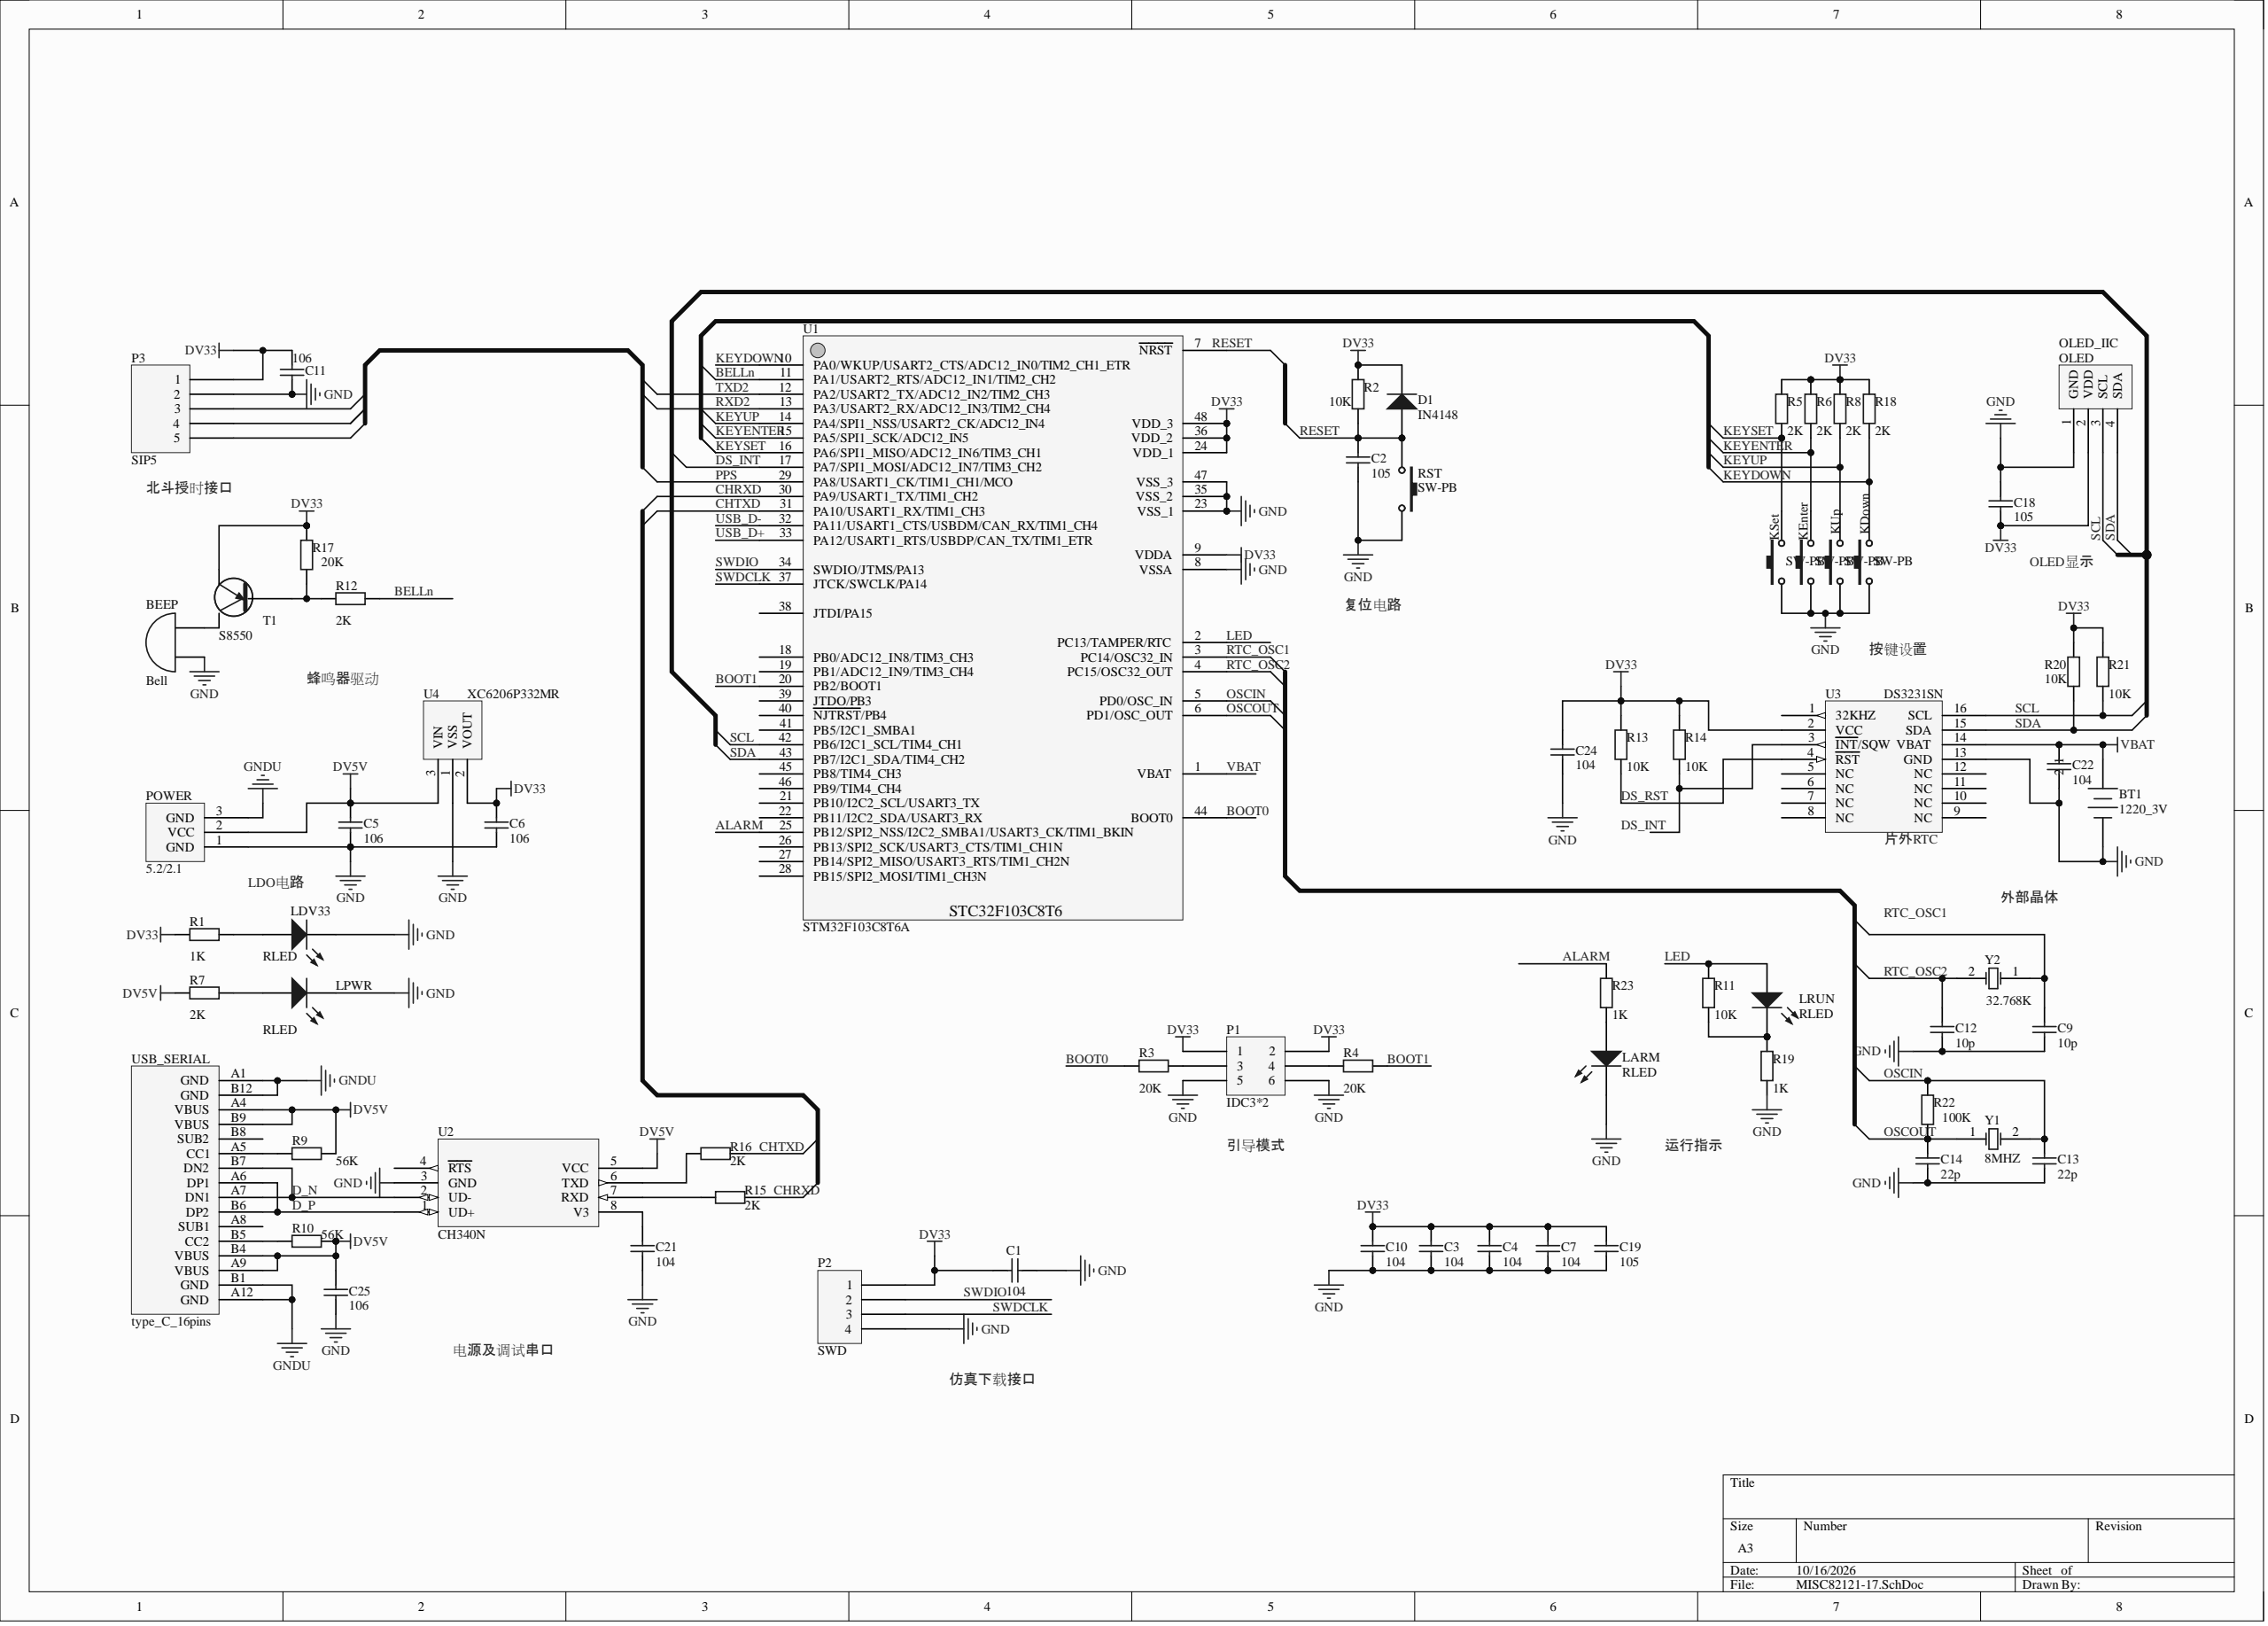Circuit board | Altium Designer | 67 parts | 42 nets
Bill of materials:
Comment,Description,Designator,Footprint,LibRef,Quantity
"Bell","Electrical Bell","BEEP","HN9650B","Bell","1"
"1220_3V","Multicell Battery","BT1","CR1220","Battery","1"
"104","Capacitor","C1, C3, C4, C7, C10, C21, C22, C24","C0805","Cap","8"
"105","Capacitor","C2, C19","C0805","Cap","2"
"106","Capacitor","C5, C6, C11","C0805","Cap","3"
"10p","Capacitor","C9, C12","C0603","Cap","2"
"22p","Capacitor","C13, C14","C0603","Cap","2"
"IN4148","Default Diode","D1","D0805","Diode","1"
"SW-PB","Switch","KDown, KEnter, KSet, KUp, RST","KEY_8mm","SW-PB","5"
"RLED","Typical INFRARED GaAs LED","LARM, LDV33, LPWR, LRUN","LED0805","LED0","4"
"OLED_IIC","","OLED","OLED","OLED_I2C_I2164","1"
"IDC3*2","","P1","HDR2X3","IDC3*2","1"
"SWD","","P2","HDR1X4","SWD","1"
"SIP5","","P3","HDR1X5","SIP5","1"
"5.2/2.1","","POWER","SWC_SET","5.2/2.1","1"
"Res2","Resistor","R1, R2, R3, R4, R5, R6, R7, R8, R9, R10, R11, R12, R13, R14, R15, R16, R17, R18, R19, R20, R21, R22, R23","R0805","Res2","23"
"S8550","","T1","SOT-23","S8550","1"
"STM32F103C8T6A","","U1","LQFP48","STM32F103C8T6","1"
"CH340N","","U2","SO-8","CH340N","1"
"DS3231SN","","U3","SOP-16","DS3231SN","1"
"XC6206P332MR","","U4","SOT-23S","XC6206P332MR","1"
"type_C_16pins","","USB_SERIAL","TYPE_C_16PIN","type_C_16pins","1"
"8MHZ","Crystal Oscillator","Y1","OSC 5032-2P","XTAL","1"
"32.768K","Crystal Oscillator","Y2","OSC_2*6","XTAL","1"
Netlist (Protel format):
[
BEEP
HN9650B
Bell



]
[
BT1
CR1220
1220_3V



]
[
C1
C0805
104



]
[
C2
C0805
105



]
[
C3
C0805
104



]
[
C4
C0805
104



]
[
C5
C0805
106



]
[
C6
C0805
106



]
[
C7
C0805
104



]
[
C9
C0603
10p



]
[
C10
C0805
104



]
[
C11
C0805
106



]
[
C12
C0603
10p



]
[
C13
C0603
22p



]
[
C14
C0603
22p



]
[
C18
C0805
105



]
[
C19
C0805
105



]
[
C21
C0805
104



]
[
C22
C0805
104



]
[
C24
C0805
104



]
[
C25
C0805
106



]
[
D1
D0805
IN4148



]
[
KDown
KEY_8mm
SW-PB



]
[
KEnter
KEY_8mm
SW-PB



]
[
KSet
KEY_8mm
SW-PB



]
[
KUp
KEY_8mm
SW-PB



]
[
LARM
LED0805
RLED



]
[
LDV33
LED0805
RLED



]
[
LPWR
LED0805
RLED



]
[
LRUN
LED0805
RLED



]
[
OLED
OLED
OLED_IIC



]
[
P1
HDR2X3
IDC3*2



]
[
P2
HDR1X4
SWD



]
[
P3
HDR1X5
SIP5



]
[
POWER
SWC_SET
5.2/2.1



]
[
R1
R0805
Res2



]
[
R2
R0805
Res2



]
[
R3
R0805
Res2



]
[
R4
R0805
Res2



]
[
R5
R0805
Res2



]
[
R6
R0805
Res2



]
[
R7
R0805
Res2



]
[
R8
R0805
Res2



]
[
R9
R0805
Res2



]
[
R10
R0805
Res2



]
[
R11
R0805
Res2



]
[
R12
R0805
Res2



]
[
R13
R0805
Res2



]
[
R14
R0805
Res2



]
[
R15
R0805
Res2



]
[
R16
R0805
Res2



]
[
R17
R0805
Res2



]
[
R18
R0805
Res2



]
[
R19
R0805
Res2



]
[
R20
R0805
Res2



]
[
R21
R0805
Res2



]
[
R22
R0805
Res2



]
[
R23
R0805
Res2



]
[
RST
KEY_8mm
SW-PB



]
[
T1
SOT-23
S8550



]
[
U1
LQFP48
STM32F103C8T6A



]
[
U2
SO-8
CH340N



]
[
U3
SOP-16
DS3231SN



]
[
U4
SOT-23S
XC6206P332MR



]
[
USB_SERIAL
TYPE_C_16PIN
type_C_16pins



]
[
Y1
OSC 5032-2P
8MHZ



]
[
Y2
OSC_2*6
32.768K



]
(
VBAT
BT1-1
C22-2
U1-1
U3-14
)
(
SWDIO
P2-2
U1-34
)
(
SWDCLK
P2-3
U1-37
)
(
SDA
OLED-4
R20-1
U1-43
U3-15
)
(
SCL
OLED-3
R21-1
U1-42
U3-16
)
(
RTC_OSC2
C12-2
U1-4
Y2-2
)
(
RESET
C2-2
D1-1
R2-1
RST-1
)
(
OSCOUT
C14-2
R22-1
U1-6
Y1-1
)
(
OSCIN
C13-2
R22-2
U1-5
Y1-2
)
(
NetR16_1
R16-1
U2-6
)
(
NetR15_1
R15-1
U2-7
)
(
NetR14_1
R14-1
U3-3
)
(
NetR12_1
R12-1
R17-1
T1-B21
)
(
NetR10_1
R10-1
USB_SERIAL-B5
)
(
NetR9_1
R9-1
USB_SERIAL-A5
)
(
NetP1_4
P1-4
R4-1
)
(
NetP1_3
P1-3
R3-2
)
(
NetLRUN_2
LRUN-2
R11-1
R19-2
)
(
NetLPWR_1
LPWR-1
R7-2
)
(
NetLDV33_1
LDV33-1
R1-2
)
(
NetLARM_1
LARM-1
R23-1
)
(
NetC21_1
C21-1
U2-8
)
(
NetC9_2
C9-2
Y2-1
)
(
NetBEEP_2
BEEP-2
T1-B20
)
(
LED
LRUN-1
R11-2
U1-2
)
(
KEYUP
KUp-2
R8-1
U1-14
)
(
KEYSET
KSet-2
R5-1
U1-16
)
(
KEYENTER
KEnter-2
R6-1
U1-15
)
(
KEYDOWN
KDown-2
R18-1
U1-10
)
(
GNDU
POWER-3
USB_SERIAL-A1
USB_SERIAL-A12
USB_SERIAL-B1
USB_SERIAL-B12
)
(
GND
BEEP-1
BT1-2
C1-2
C2-1
C3-1
C4-1
C5-1
C6-1
C7-1
C9-1
C10-1
C11-1
C12-1
C13-1
C14-1
C18-2
C19-1
C21-2
C22-1
C24-1
C25-1
KDown-1
KEnter-1
KSet-1
KUp-1
LARM-2
LDV33-2
LPWR-2
OLED-1
P1-5
P1-6
P2-4
P3-B27
POWER-1
R19-1
RST-2
U1-8
U1-23
U1-35
U1-47
U2-3
U3-13
U4-1
)
(
DV33
C1-1
C3-2
C4-2
C6-2
C7-2
C10-2
C11-2
C18-1
C19-2
C24-2
D1-2
OLED-2
P1-1
P1-2
P2-1
P3-B28
R1-1
R2-2
R5-2
R6-2
R8-2
R13-2
R14-2
R17-2
R18-2
R20-2
R21-2
T1-B19
U1-9
U1-24
U1-36
U1-48
U3-2
U4-2
)
(
DV5V
C5-2
C25-2
POWER-2
R7-1
R9-2
R10-2
U2-5
U4-3
USB_SERIAL-A4
USB_SERIAL-A9
USB_SERIAL-B4
USB_SERIAL-B9
)
(
DS_RST
R13-1
U3-4
)
(
D_P
U2-1
USB_SERIAL-A6
USB_SERIAL-B6
)
(
D_N
U2-2
USB_SERIAL-A7
USB_SERIAL-B7
)
(
CHTXD
R16-2
U1-31
)
(
CHRXD
R15-2
U1-30
)
(
BOOT1
R4-2
U1-20
)
(
BOOT0
R3-1
U1-44
)
(
BELLn
R12-2
U1-11
)
(
ALARM
R23-2
U1-25
)